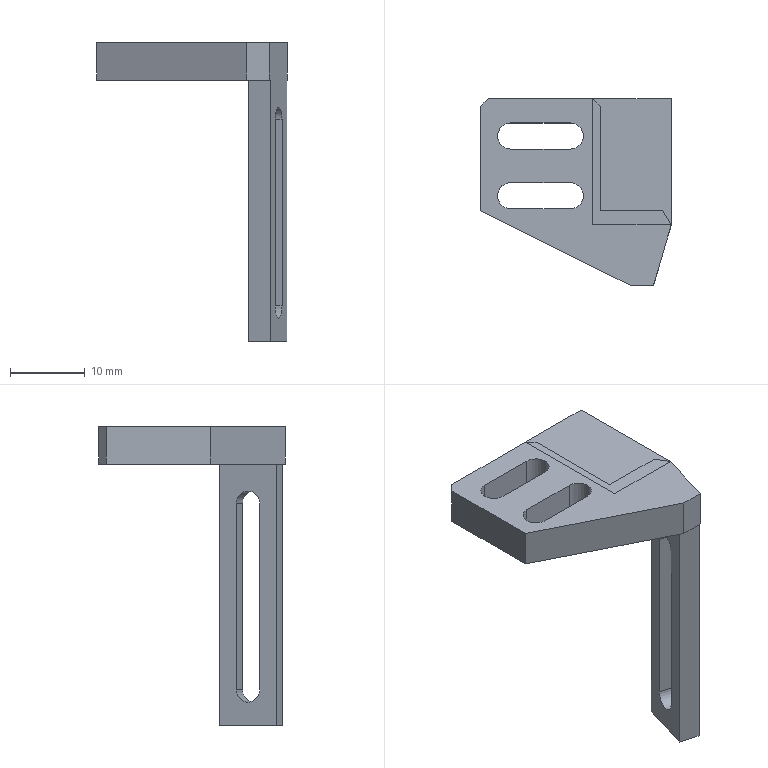NC program | NX | posted with a generic post | part box 25.523 x 25 x 40 mm
Whole program:
N10 G17 G21 G94 G90
(FLOOR_WALL_COPY , TOOL : D63)
N12 T03 M6
N14 G54
N16 G17 G0 G90 X59.5 Y12.761 B0. C0. S6500 M3
N18 G43 Z30. H3
N20 Z7.
N22 G94 G1 Z4. F1500.
N24 X56.5
N26 X-31.5
N28 X-34.5
N30 Z7.
N32 G0 Z30.
N34 X59.5
N36 Z6.
N38 G1 Z3.
N40 X56.5
N42 X-31.5
N44 X-34.5
N46 Z6.
N48 G0 Z30.
N50 X59.5
N52 Z5.
N54 G1 Z2.
N56 X56.5
N58 X-31.5
N60 X-34.5
N62 Z5.
N64 G0 Z30.
N66 X59.5
N68 Z4.
N70 G1 Z1.
N72 X56.5
N74 X-31.5
N76 X-34.5
N78 Z4.
N80 G0 Z30.
N82 X59.5
N84 Z3.
N86 G1 Z0.
N88 X56.5
N90 X-31.5
N92 X-34.5
N94 Z3.
N96 G0 Z30.
N98 M5
N100 M2